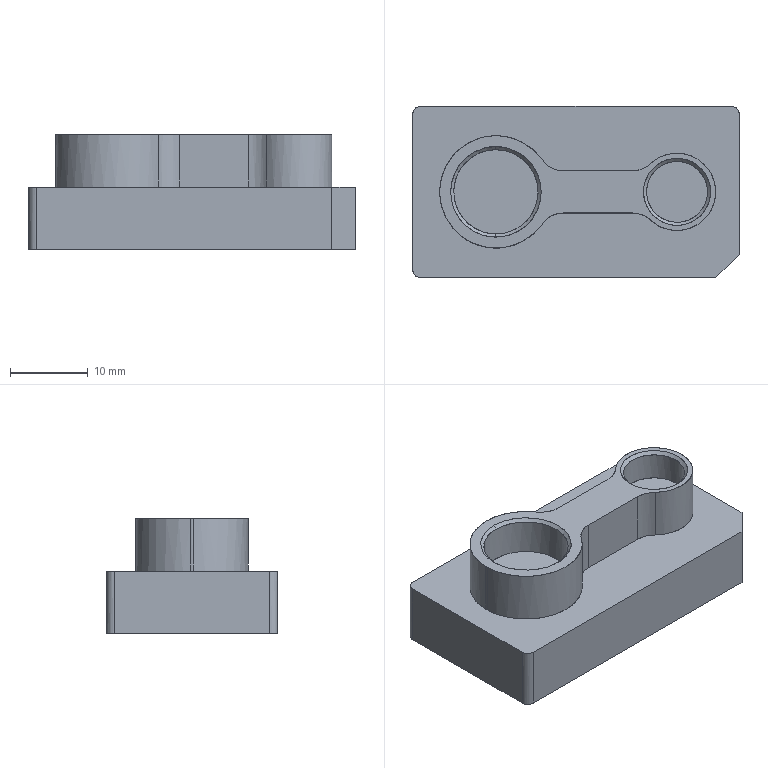CAM job | PowerMill | 3-axis milling, other | part box 42 x 22 x 14.721 mm
Tools:
number,name,type,diameter,tip_radius,length,cutting_length,overhang,flutes,holder,toolpaths_using
1,D10C,end_mill,10.0,0.0,60.0,,30.0,1,D42L35,1
4,R1_1,ball_nosed,2.0,1.0,3.0,,2.0,1,D42L35,1
1,D10C_1_1,end_mill,10.0,0.0,60.0,,15.16,1,D42L35,3
2,D4C_1_1,end_mill,4.0,0.0,30.0,,6.92,1,D42L35,1
3,D10_1_1,end_mill,10.0,0.0,60.0,,14.88,1,D42L35,3
14,D4_1_1_1,end_mill,4.0,0.0,30.0,,7.0,1,D42L35,2
13,Text_D4_1_1,taper_spherical,4.0,0.3,60.0,,7.0,1,D42L35,1
Operations:
program,toolpath,strategy,tool,tool_number,tool_diameter,tip_radius,flutes,spindle_rpm,feed_cut,surface_speed_m_min_computed,feed_per_tooth_computed,tolerance,thickness,stepover,stepdown,cut_length,cut_time_min,total_time_min,workplane
04-0505-1-F,精公开粗01-扫面平行-D10C,raster_area_clear,D10C_1_1,1,10.0,0.0,1.0,8000.0,10000.0,251.33,1.25,0.03,0.28,6.0,1.0,312.92,0.031,0.0376,
04-0505-1-F,精公开粗01-外形偏置-D10C,offset_area_clear,D10C_1_1,1,10.0,0.0,1.0,8000.0,10000.0,251.33,1.25,0.03,0.28,6.0,1.0,4883.606,0.488,0.5333,
04-0505-1-F,精公开粗01-基准台等高-D10C,constantz,D10C_1_1,1,10.0,0.0,1.0,8000.0,10000.0,251.33,1.25,0.03,0.07,5.0,0.4,3449.072,0.345,0.3541,
04-0505-1-F,精公再粗02-外形偏置-D4C,offset_area_clear,D4C_1_1,2,4.0,0.0,1.0,18000.0,6000.0,226.19,0.3333,0.03,0.0,2.0,1.0,5040.649,0.84,1.108,
04-0505-1-F,精公基准台01-平坦面平行-D10,raster_area_clear,D10_1_1,3,10.0,0.0,1.0,8500.0,600.0,267.04,0.0706,0.005,0.38,5.0,1.0,232.895,0.388,0.405,
04-0505-1-F,精公基准台01-基准面偏置-D10,offset_area_clear,D10_1_1,3,10.0,0.0,1.0,8500.0,600.0,267.04,0.0706,0.005,0.38,5.0,1.0,133.001,0.222,0.2396,
04-0505-1-F,精公基准台01-基准台侧光-D10,profile_area_clear,D10_1_1,3,10.0,0.0,1.0,8500.0,600.0,267.04,0.0706,0.005,0.0,0.08,1.0,313.233,0.522,0.5858,
04-0505-1-F,精公精光01-平行-R1,raster,R1_1,4,2.0,1.0,1.0,18000.0,2000.0,113.1,0.1111,0.005,-0.075,0.03,1.0,1471.512,0.736,0.7776,
04-0505-1-F,精公精光02-平坦面偏置-D4,offset_area_clear,D4_1_1_1,14,4.0,0.0,1.0,18000.0,600.0,226.19,0.0333,0.005,0.375,2.0,1.0,277.695,0.463,0.5289,
04-0505-1-F,精公精光02-等高-D4,constantz,D4_1_1_1,14,4.0,0.0,1.0,18000.0,2000.0,226.19,0.1111,0.005,-0.075,5.0,0.1,8569.34,4.285,4.299,
04-0505-1-F,精公刻字01-刻字-Text_D4,pattern,Text_D4_1_1,13,4.0,0.3,1.0,15000.0,1000.0,188.5,0.0667,0.005,0.0,5.0,1.0,43.043,0.043,0.0599,
,精公开粗01-外形偏置-D10C_Reference,offset_area_clear,D10C,1,10.0,0.0,1.0,8000.0,10000.0,251.33,1.25,0.03,0.28,6.0,1.0,9766.783,0.977,1.063,